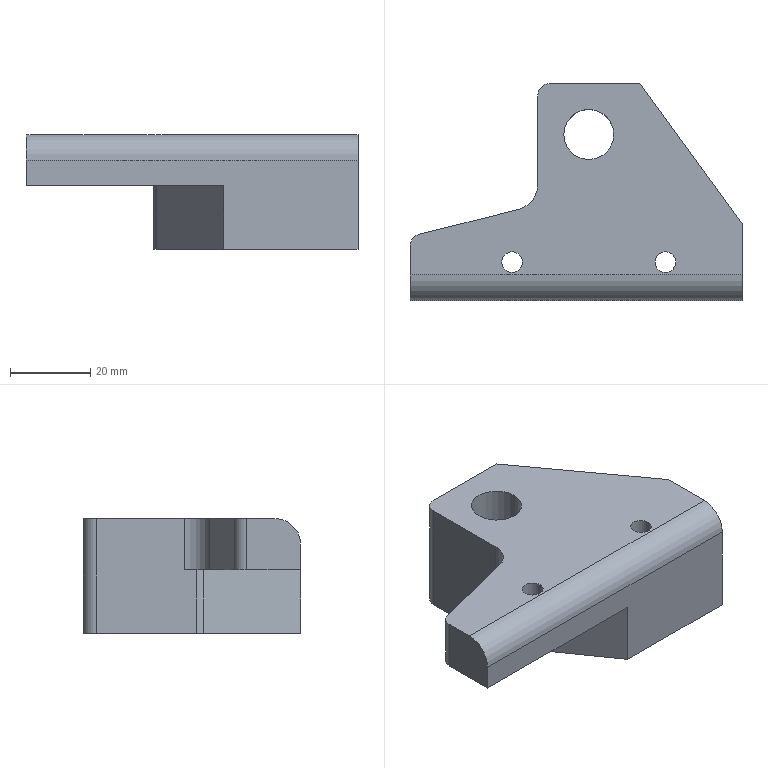Part | NX | 1 solid | 32 faces | box 82.55 x 53.975 x 28.575 mm | volume 59843 mm3 | cylinder 17 | plane 13 | cone 2 | commonest cylinder face diameters 5.16 x4 15.875 x4 6.35 x3 4.915 x2 12.446 x2 12.7 x2
STEP:
#1=CARTESIAN_POINT('',(-7.938,-17.462,0.));
#2=VERTEX_POINT('',#1);
#3=CARTESIAN_POINT('',(-23.812,-17.462,0.));
#4=VERTEX_POINT('',#3);
#5=CARTESIAN_POINT('',(-15.875,-17.462,0.));
#6=DIRECTION('',(0.,0.,-1.));
#7=DIRECTION('',(-1.,0.,0.));
#8=AXIS2_PLACEMENT_3D('',#5,#6,#7);
#9=CIRCLE('',#8,7.938);
#10=EDGE_CURVE('',#2,#4,#9,.T.);
#11=ORIENTED_EDGE('',*,*,#10,.F.);
#12=CARTESIAN_POINT('',(-7.938,-17.462,-6.35));
#13=VERTEX_POINT('',#12);
#14=CARTESIAN_POINT('',(-7.938,-17.462,0.));
#15=DIRECTION('',(0.,0.,-1.));
#16=VECTOR('',#15,1000.);
#17=LINE('',#14,#16);
#18=EDGE_CURVE('',#2,#13,#17,.T.);
#19=ORIENTED_EDGE('',*,*,#18,.T.);
#20=CARTESIAN_POINT('',(-23.812,-17.462,-6.35));
#21=VERTEX_POINT('',#20);
#22=CARTESIAN_POINT('',(-15.875,-17.462,-6.35));
#23=DIRECTION('',(0.,0.,-1.));
#24=DIRECTION('',(-1.,0.,0.));
#25=AXIS2_PLACEMENT_3D('',#22,#23,#24);
#26=CIRCLE('',#25,7.938);
#27=EDGE_CURVE('',#13,#21,#26,.T.);
#28=ORIENTED_EDGE('',*,*,#27,.T.);
#29=CARTESIAN_POINT('',(-23.812,-17.462,0.));
#30=DIRECTION('',(0.,0.,-1.));
#31=VECTOR('',#30,1000.);
#32=LINE('',#29,#31);
#33=EDGE_CURVE('',#4,#21,#32,.T.);
#34=ORIENTED_EDGE('',*,*,#33,.F.);
#35=EDGE_LOOP('',(#11,#19,#28,#34));
#36=FACE_BOUND('',#35,.T.);
#37=CARTESIAN_POINT('',(-15.875,-17.462,0.));
#38=DIRECTION('',(0.,0.,-1.));
#39=DIRECTION('',(1.,0.,0.));
#40=AXIS2_PLACEMENT_3D('',#37,#38,#39);
#41=CYLINDRICAL_SURFACE('',#40,7.938);
#42=ADVANCED_FACE('',(#36),#41,.F.);
#43=CARTESIAN_POINT('',(30.163,-17.462,0.));
#44=VERTEX_POINT('',#43);
#45=CARTESIAN_POINT('',(14.287,-17.462,0.));
#46=VERTEX_POINT('',#45);
#47=CARTESIAN_POINT('',(22.225,-17.462,0.));
#48=DIRECTION('',(0.,0.,-1.));
#49=DIRECTION('',(-1.,0.,0.));
#50=AXIS2_PLACEMENT_3D('',#47,#48,#49);
#51=CIRCLE('',#50,7.938);
#52=EDGE_CURVE('',#44,#46,#51,.T.);
#53=ORIENTED_EDGE('',*,*,#52,.F.);
#54=CARTESIAN_POINT('',(30.163,-17.462,-22.225));
#55=VERTEX_POINT('',#54);
#56=CARTESIAN_POINT('',(30.163,-17.462,0.));
#57=DIRECTION('',(0.,0.,-1.));
#58=VECTOR('',#57,1000.);
#59=LINE('',#56,#58);
#60=EDGE_CURVE('',#44,#55,#59,.T.);
#61=ORIENTED_EDGE('',*,*,#60,.T.);
#62=CARTESIAN_POINT('',(14.287,-17.462,-22.225));
#63=VERTEX_POINT('',#62);
#64=CARTESIAN_POINT('',(22.225,-17.462,-22.225));
#65=DIRECTION('',(0.,0.,-1.));
#66=DIRECTION('',(-1.,0.,0.));
#67=AXIS2_PLACEMENT_3D('',#64,#65,#66);
#68=CIRCLE('',#67,7.938);
#69=EDGE_CURVE('',#55,#63,#68,.T.);
#70=ORIENTED_EDGE('',*,*,#69,.T.);
#71=CARTESIAN_POINT('',(14.287,-17.462,0.));
#72=DIRECTION('',(0.,0.,-1.));
#73=VECTOR('',#72,1000.);
#74=LINE('',#71,#73);
#75=EDGE_CURVE('',#46,#63,#74,.T.);
#76=ORIENTED_EDGE('',*,*,#75,.F.);
#77=EDGE_LOOP('',(#53,#61,#70,#76));
#78=FACE_BOUND('',#77,.T.);
#79=CARTESIAN_POINT('',(22.225,-17.462,0.));
#80=DIRECTION('',(0.,0.,-1.));
#81=DIRECTION('',(1.,0.,0.));
#82=AXIS2_PLACEMENT_3D('',#79,#80,#81);
#83=CYLINDRICAL_SURFACE('',#82,7.938);
#84=ADVANCED_FACE('',(#78),#83,.F.);
#85=CARTESIAN_POINT('',(30.15,-1.587,-8.048));
#86=VERTEX_POINT('',#85);
#87=CARTESIAN_POINT('',(27.692,-1.587,-9.525));
#88=VERTEX_POINT('',#87);
#89=CARTESIAN_POINT('',(27.692,-1.587,-9.525));
#90=DIRECTION('',(-0.8572,0.,-0.515));
#91=VECTOR('',#90,1000.);
#92=LINE('',#89,#91);
#93=EDGE_CURVE('',#86,#88,#92,.T.);
#94=ORIENTED_EDGE('',*,*,#93,.F.);
#95=CARTESIAN_POINT('',(32.607,-1.587,-9.525));
#96=VERTEX_POINT('',#95);
#97=CARTESIAN_POINT('',(32.607,-1.587,-9.525));
#98=DIRECTION('',(0.8572,0.,-0.515));
#99=VECTOR('',#98,1000.);
#100=LINE('',#97,#99);
#101=EDGE_CURVE('',#86,#96,#100,.T.);
#102=ORIENTED_EDGE('',*,*,#101,.T.);
#103=CARTESIAN_POINT('',(30.15,-1.587,-9.525));
#104=DIRECTION('',(0.,0.,-1.));
#105=DIRECTION('',(-1.,0.,0.));
#106=AXIS2_PLACEMENT_3D('',#103,#104,#105);
#107=CIRCLE('',#106,2.457);
#108=EDGE_CURVE('',#96,#88,#107,.T.);
#109=ORIENTED_EDGE('',*,*,#108,.T.);
#110=EDGE_LOOP('',(#94,#102,#109));
#111=FACE_BOUND('',#110,.T.);
#112=CARTESIAN_POINT('',(30.15,-1.587,-9.525));
#113=DIRECTION('',(0.,0.,-1.));
#114=DIRECTION('',(1.,0.,0.));
#115=AXIS2_PLACEMENT_3D('',#112,#113,#114);
#116=CONICAL_SURFACE('',#115,2.457,1.03);
#117=ADVANCED_FACE('',(#111),#116,.F.);
#118=ORIENTED_EDGE('',*,*,#108,.F.);
#119=CARTESIAN_POINT('',(32.607,-1.587,-22.225));
#120=VERTEX_POINT('',#119);
#121=CARTESIAN_POINT('',(32.607,-1.587,-22.225));
#122=DIRECTION('',(0.,0.,-1.));
#123=VECTOR('',#122,1000.);
#124=LINE('',#121,#123);
#125=EDGE_CURVE('',#96,#120,#124,.T.);
#126=ORIENTED_EDGE('',*,*,#125,.T.);
#127=CARTESIAN_POINT('',(27.692,-1.587,-22.225));
#128=VERTEX_POINT('',#127);
#129=CARTESIAN_POINT('',(30.15,-1.587,-22.225));
#130=DIRECTION('',(0.,0.,-1.));
#131=DIRECTION('',(-1.,0.,0.));
#132=AXIS2_PLACEMENT_3D('',#129,#130,#131);
#133=CIRCLE('',#132,2.457);
#134=EDGE_CURVE('',#120,#128,#133,.T.);
#135=ORIENTED_EDGE('',*,*,#134,.T.);
#136=CARTESIAN_POINT('',(27.692,-1.587,-22.225));
#137=DIRECTION('',(0.,0.,-1.));
#138=VECTOR('',#137,1000.);
#139=LINE('',#136,#138);
#140=EDGE_CURVE('',#88,#128,#139,.T.);
#141=ORIENTED_EDGE('',*,*,#140,.F.);
#142=EDGE_LOOP('',(#118,#126,#135,#141));
#143=FACE_BOUND('',#142,.T.);
#144=CARTESIAN_POINT('',(30.15,-1.587,-22.225));
#145=DIRECTION('',(0.,0.,-1.));
#146=DIRECTION('',(1.,0.,0.));
#147=AXIS2_PLACEMENT_3D('',#144,#145,#146);
#148=CYLINDRICAL_SURFACE('',#147,2.457);
#149=ADVANCED_FACE('',(#143),#148,.F.);
#150=CARTESIAN_POINT('',(9.398,14.287,6.35));
#151=VERTEX_POINT('',#150);
#152=CARTESIAN_POINT('',(-3.048,14.287,6.35));
#153=VERTEX_POINT('',#152);
#154=CARTESIAN_POINT('',(3.175,14.287,6.35));
#155=DIRECTION('',(0.,0.,-1.));
#156=DIRECTION('',(-1.,0.,0.));
#157=AXIS2_PLACEMENT_3D('',#154,#155,#156);
#158=CIRCLE('',#157,6.223);
#159=EDGE_CURVE('',#151,#153,#158,.T.);
#160=ORIENTED_EDGE('',*,*,#159,.F.);
#161=CARTESIAN_POINT('',(9.398,14.287,-22.225));
#162=VERTEX_POINT('',#161);
#163=CARTESIAN_POINT('',(9.398,14.287,6.35));
#164=DIRECTION('',(0.,0.,-1.));
#165=VECTOR('',#164,1000.);
#166=LINE('',#163,#165);
#167=EDGE_CURVE('',#151,#162,#166,.T.);
#168=ORIENTED_EDGE('',*,*,#167,.T.);
#169=CARTESIAN_POINT('',(-3.048,14.287,-22.225));
#170=VERTEX_POINT('',#169);
#171=CARTESIAN_POINT('',(3.175,14.287,-22.225));
#172=DIRECTION('',(0.,0.,-1.));
#173=DIRECTION('',(-1.,0.,0.));
#174=AXIS2_PLACEMENT_3D('',#171,#172,#173);
#175=CIRCLE('',#174,6.223);
#176=EDGE_CURVE('',#162,#170,#175,.T.);
#177=ORIENTED_EDGE('',*,*,#176,.T.);
#178=CARTESIAN_POINT('',(-3.048,14.287,6.35));
#179=DIRECTION('',(0.,0.,-1.));
#180=VECTOR('',#179,1000.);
#181=LINE('',#178,#180);
#182=EDGE_CURVE('',#153,#170,#181,.T.);
#183=ORIENTED_EDGE('',*,*,#182,.F.);
#184=EDGE_LOOP('',(#160,#168,#177,#183));
#185=FACE_BOUND('',#184,.T.);
#186=CARTESIAN_POINT('',(3.175,14.287,6.35));
#187=DIRECTION('',(0.,0.,-1.));
#188=DIRECTION('',(1.,0.,0.));
#189=AXIS2_PLACEMENT_3D('',#186,#187,#188);
#190=CYLINDRICAL_SURFACE('',#189,6.223);
#191=ADVANCED_FACE('',(#185),#190,.F.);
#192=CARTESIAN_POINT('',(24.805,-17.462,6.35));
#193=VERTEX_POINT('',#192);
#194=CARTESIAN_POINT('',(19.645,-17.462,6.35));
#195=VERTEX_POINT('',#194);
#196=CARTESIAN_POINT('',(22.225,-17.462,6.35));
#197=DIRECTION('',(0.,0.,-1.));
#198=DIRECTION('',(-1.,0.,0.));
#199=AXIS2_PLACEMENT_3D('',#196,#197,#198);
#200=CIRCLE('',#199,2.58);
#201=EDGE_CURVE('',#193,#195,#200,.T.);
#202=ORIENTED_EDGE('',*,*,#201,.F.);
#203=CARTESIAN_POINT('',(24.805,-17.462,0.));
#204=VERTEX_POINT('',#203);
#205=CARTESIAN_POINT('',(24.805,-17.462,-22.225));
#206=DIRECTION('',(0.,0.,-1.));
#207=VECTOR('',#206,1000.);
#208=LINE('',#205,#207);
#209=EDGE_CURVE('',#193,#204,#208,.T.);
#210=ORIENTED_EDGE('',*,*,#209,.T.);
#211=CARTESIAN_POINT('',(19.645,-17.462,0.));
#212=VERTEX_POINT('',#211);
#213=CARTESIAN_POINT('',(22.225,-17.462,0.));
#214=DIRECTION('',(0.,0.,1.));
#215=DIRECTION('',(-1.,0.,0.));
#216=AXIS2_PLACEMENT_3D('',#213,#214,#215);
#217=CIRCLE('',#216,2.58);
#218=EDGE_CURVE('',#212,#204,#217,.T.);
#219=ORIENTED_EDGE('',*,*,#218,.F.);
#220=CARTESIAN_POINT('',(19.645,-17.462,-22.225));
#221=DIRECTION('',(0.,0.,-1.));
#222=VECTOR('',#221,1000.);
#223=LINE('',#220,#222);
#224=EDGE_CURVE('',#195,#212,#223,.T.);
#225=ORIENTED_EDGE('',*,*,#224,.F.);
#226=EDGE_LOOP('',(#202,#210,#219,#225));
#227=FACE_BOUND('',#226,.T.);
#228=CARTESIAN_POINT('',(22.225,-17.462,-22.225));
#229=DIRECTION('',(0.,0.,-1.));
#230=DIRECTION('',(1.,0.,0.));
#231=AXIS2_PLACEMENT_3D('',#228,#229,#230);
#232=CYLINDRICAL_SURFACE('',#231,2.58);
#233=ADVANCED_FACE('',(#227),#232,.F.);
#234=CARTESIAN_POINT('',(-13.295,-17.462,6.35));
#235=VERTEX_POINT('',#234);
#236=CARTESIAN_POINT('',(-18.455,-17.462,6.35));
#237=VERTEX_POINT('',#236);
#238=CARTESIAN_POINT('',(-15.875,-17.462,6.35));
#239=DIRECTION('',(0.,0.,-1.));
#240=DIRECTION('',(-1.,0.,0.));
#241=AXIS2_PLACEMENT_3D('',#238,#239,#240);
#242=CIRCLE('',#241,2.58);
#243=EDGE_CURVE('',#235,#237,#242,.T.);
#244=ORIENTED_EDGE('',*,*,#243,.F.);
#245=CARTESIAN_POINT('',(-13.295,-17.462,0.));
#246=VERTEX_POINT('',#245);
#247=CARTESIAN_POINT('',(-13.295,-17.462,-22.225));
#248=DIRECTION('',(0.,0.,-1.));
#249=VECTOR('',#248,1000.);
#250=LINE('',#247,#249);
#251=EDGE_CURVE('',#235,#246,#250,.T.);
#252=ORIENTED_EDGE('',*,*,#251,.T.);
#253=CARTESIAN_POINT('',(-18.455,-17.462,0.));
#254=VERTEX_POINT('',#253);
#255=CARTESIAN_POINT('',(-15.875,-17.462,0.));
#256=DIRECTION('',(0.,0.,1.));
#257=DIRECTION('',(-1.,0.,0.));
#258=AXIS2_PLACEMENT_3D('',#255,#256,#257);
#259=CIRCLE('',#258,2.58);
#260=EDGE_CURVE('',#254,#246,#259,.T.);
#261=ORIENTED_EDGE('',*,*,#260,.F.);
#262=CARTESIAN_POINT('',(-18.455,-17.462,-22.225));
#263=DIRECTION('',(0.,0.,-1.));
#264=VECTOR('',#263,1000.);
#265=LINE('',#262,#264);
#266=EDGE_CURVE('',#237,#254,#265,.T.);
#267=ORIENTED_EDGE('',*,*,#266,.F.);
#268=EDGE_LOOP('',(#244,#252,#261,#267));
#269=FACE_BOUND('',#268,.T.);
#270=CARTESIAN_POINT('',(-15.875,-17.462,-22.225));
#271=DIRECTION('',(0.,0.,-1.));
#272=DIRECTION('',(1.,0.,0.));
#273=AXIS2_PLACEMENT_3D('',#270,#271,#272);
#274=CYLINDRICAL_SURFACE('',#273,2.58);
#275=ADVANCED_FACE('',(#269),#274,.F.);
#276=ORIENTED_EDGE('',*,*,#251,.F.);
#277=CARTESIAN_POINT('',(-15.875,-17.462,6.35));
#278=DIRECTION('',(0.,0.,-1.));
#279=DIRECTION('',(-1.,0.,0.));
#280=AXIS2_PLACEMENT_3D('',#277,#278,#279);
#281=CIRCLE('',#280,2.58);
#282=EDGE_CURVE('',#237,#235,#281,.T.);
#283=ORIENTED_EDGE('',*,*,#282,.F.);
#284=ORIENTED_EDGE('',*,*,#266,.T.);
#285=CARTESIAN_POINT('',(-15.875,-17.462,0.));
#286=DIRECTION('',(0.,0.,1.));
#287=DIRECTION('',(-1.,0.,0.));
#288=AXIS2_PLACEMENT_3D('',#285,#286,#287);
#289=CIRCLE('',#288,2.58);
#290=EDGE_CURVE('',#246,#254,#289,.T.);
#291=ORIENTED_EDGE('',*,*,#290,.F.);
#292=EDGE_LOOP('',(#276,#283,#284,#291));
#293=FACE_BOUND('',#292,.T.);
#294=CARTESIAN_POINT('',(-15.875,-17.462,-22.225));
#295=DIRECTION('',(0.,0.,-1.));
#296=DIRECTION('',(1.,0.,0.));
#297=AXIS2_PLACEMENT_3D('',#294,#295,#296);
#298=CYLINDRICAL_SURFACE('',#297,2.58);
#299=ADVANCED_FACE('',(#293),#298,.F.);
#300=ORIENTED_EDGE('',*,*,#209,.F.);
#301=CARTESIAN_POINT('',(22.225,-17.462,6.35));
#302=DIRECTION('',(0.,0.,-1.));
#303=DIRECTION('',(-1.,0.,0.));
#304=AXIS2_PLACEMENT_3D('',#301,#302,#303);
#305=CIRCLE('',#304,2.58);
#306=EDGE_CURVE('',#195,#193,#305,.T.);
#307=ORIENTED_EDGE('',*,*,#306,.F.);
#308=ORIENTED_EDGE('',*,*,#224,.T.);
#309=CARTESIAN_POINT('',(22.225,-17.462,0.));
#310=DIRECTION('',(0.,0.,1.));
#311=DIRECTION('',(-1.,0.,0.));
#312=AXIS2_PLACEMENT_3D('',#309,#310,#311);
#313=CIRCLE('',#312,2.58);
#314=EDGE_CURVE('',#204,#212,#313,.T.);
#315=ORIENTED_EDGE('',*,*,#314,.F.);
#316=EDGE_LOOP('',(#300,#307,#308,#315));
#317=FACE_BOUND('',#316,.T.);
#318=CARTESIAN_POINT('',(22.225,-17.462,-22.225));
#319=DIRECTION('',(0.,0.,-1.));
#320=DIRECTION('',(1.,0.,0.));
#321=AXIS2_PLACEMENT_3D('',#318,#319,#320);
#322=CYLINDRICAL_SURFACE('',#321,2.58);
#323=ADVANCED_FACE('',(#317),#322,.F.);
#324=CARTESIAN_POINT('',(41.275,-7.938,6.35));
#325=VERTEX_POINT('',#324);
#326=CARTESIAN_POINT('',(41.275,-7.938,-22.225));
#327=VERTEX_POINT('',#326);
#328=CARTESIAN_POINT('',(41.275,-7.938,6.35));
#329=DIRECTION('',(0.,0.,-1.));
#330=VECTOR('',#329,1000.);
#331=LINE('',#328,#330);
#332=EDGE_CURVE('',#325,#327,#331,.T.);
#333=ORIENTED_EDGE('',*,*,#332,.T.);
#334=CARTESIAN_POINT('',(15.875,26.988,-22.225));
#335=VERTEX_POINT('',#334);
#336=CARTESIAN_POINT('',(41.275,-7.938,-22.225));
#337=DIRECTION('',(-0.5882,0.8087,0.));
#338=VECTOR('',#337,1000.);
#339=LINE('',#336,#338);
#340=EDGE_CURVE('',#327,#335,#339,.T.);
#341=ORIENTED_EDGE('',*,*,#340,.T.);
#342=CARTESIAN_POINT('',(15.875,26.988,6.35));
#343=VERTEX_POINT('',#342);
#344=CARTESIAN_POINT('',(15.875,26.988,6.35));
#345=DIRECTION('',(0.,0.,-1.));
#346=VECTOR('',#345,1000.);
#347=LINE('',#344,#346);
#348=EDGE_CURVE('',#343,#335,#347,.T.);
#349=ORIENTED_EDGE('',*,*,#348,.F.);
#350=CARTESIAN_POINT('',(41.275,-7.938,6.35));
#351=DIRECTION('',(-0.5882,0.8087,0.));
#352=VECTOR('',#351,1000.);
#353=LINE('',#350,#352);
#354=EDGE_CURVE('',#325,#343,#353,.T.);
#355=ORIENTED_EDGE('',*,*,#354,.F.);
#356=EDGE_LOOP('',(#333,#341,#349,#355));
#357=FACE_BOUND('',#356,.T.);
#358=CARTESIAN_POINT('',(41.275,-7.938,6.35));
#359=DIRECTION('',(-0.8087,-0.5882,0.));
#360=DIRECTION('',(-0.5882,0.8087,0.));
#361=AXIS2_PLACEMENT_3D('',#358,#359,#360);
#362=PLANE('',#361);
#363=ADVANCED_FACE('',(#357),#362,.F.);
#364=ORIENTED_EDGE('',*,*,#348,.T.);
#365=CARTESIAN_POINT('',(-6.35,26.988,-22.225));
#366=VERTEX_POINT('',#365);
#367=CARTESIAN_POINT('',(15.875,26.988,-22.225));
#368=DIRECTION('',(-1.,0.,0.));
#369=VECTOR('',#368,1000.);
#370=LINE('',#367,#369);
#371=EDGE_CURVE('',#335,#366,#370,.T.);
#372=ORIENTED_EDGE('',*,*,#371,.T.);
#373=CARTESIAN_POINT('',(-6.35,26.988,6.35));
#374=VERTEX_POINT('',#373);
#375=CARTESIAN_POINT('',(-6.35,26.988,6.35));
#376=DIRECTION('',(0.,0.,1.));
#377=VECTOR('',#376,1000.);
#378=LINE('',#375,#377);
#379=EDGE_CURVE('',#366,#374,#378,.T.);
#380=ORIENTED_EDGE('',*,*,#379,.T.);
#381=CARTESIAN_POINT('',(15.875,26.988,6.35));
#382=DIRECTION('',(-1.,0.,0.));
#383=VECTOR('',#382,1000.);
#384=LINE('',#381,#383);
#385=EDGE_CURVE('',#343,#374,#384,.T.);
#386=ORIENTED_EDGE('',*,*,#385,.F.);
#387=EDGE_LOOP('',(#364,#372,#380,#386));
#388=FACE_BOUND('',#387,.T.);
#389=CARTESIAN_POINT('',(15.875,26.988,6.35));
#390=DIRECTION('',(0.,-1.,0.));
#391=DIRECTION('',(-1.,0.,0.));
#392=AXIS2_PLACEMENT_3D('',#389,#390,#391);
#393=PLANE('',#392);
#394=ADVANCED_FACE('',(#388),#393,.F.);
#395=CARTESIAN_POINT('',(-9.525,23.812,6.35));
#396=VERTEX_POINT('',#395);
#397=CARTESIAN_POINT('',(-9.525,23.812,-22.225));
#398=VERTEX_POINT('',#397);
#399=CARTESIAN_POINT('',(-9.525,23.812,6.35));
#400=DIRECTION('',(0.,0.,-1.));
#401=VECTOR('',#400,1000.);
#402=LINE('',#399,#401);
#403=EDGE_CURVE('',#396,#398,#402,.T.);
#404=ORIENTED_EDGE('',*,*,#403,.T.);
#405=CARTESIAN_POINT('',(-9.525,-1.047,-22.225));
#406=VERTEX_POINT('',#405);
#407=CARTESIAN_POINT('',(-9.525,23.812,-22.225));
#408=DIRECTION('',(0.,-1.,0.));
#409=VECTOR('',#408,1000.);
#410=LINE('',#407,#409);
#411=EDGE_CURVE('',#398,#406,#410,.T.);
#412=ORIENTED_EDGE('',*,*,#411,.T.);
#413=CARTESIAN_POINT('',(-9.525,-1.047,-6.35));
#414=VERTEX_POINT('',#413);
#415=CARTESIAN_POINT('',(-9.525,-1.047,-22.225));
#416=DIRECTION('',(0.,0.,1.));
#417=VECTOR('',#416,1000.);
#418=LINE('',#415,#417);
#419=EDGE_CURVE('',#406,#414,#418,.T.);
#420=ORIENTED_EDGE('',*,*,#419,.T.);
#421=CARTESIAN_POINT('',(-9.525,1.794,-6.35));
#422=VERTEX_POINT('',#421);
#423=CARTESIAN_POINT('',(-9.525,6.863,-6.35));
#424=DIRECTION('',(0.,-1.,0.));
#425=VECTOR('',#424,1000.);
#426=LINE('',#423,#425);
#427=EDGE_CURVE('',#422,#414,#426,.T.);
#428=ORIENTED_EDGE('',*,*,#427,.F.);
#429=CARTESIAN_POINT('',(-9.525,1.794,6.35));
#430=VERTEX_POINT('',#429);
#431=CARTESIAN_POINT('',(-9.525,1.794,6.35));
#432=DIRECTION('',(0.,0.,1.));
#433=VECTOR('',#432,1000.);
#434=LINE('',#431,#433);
#435=EDGE_CURVE('',#422,#430,#434,.T.);
#436=ORIENTED_EDGE('',*,*,#435,.T.);
#437=CARTESIAN_POINT('',(-9.525,26.988,6.35));
#438=DIRECTION('',(0.,-1.,0.));
#439=VECTOR('',#438,1000.);
#440=LINE('',#437,#439);
#441=EDGE_CURVE('',#396,#430,#440,.T.);
#442=ORIENTED_EDGE('',*,*,#441,.F.);
#443=EDGE_LOOP('',(#404,#412,#420,#428,#436,#442));
#444=FACE_BOUND('',#443,.T.);
#445=CARTESIAN_POINT('',(-9.525,26.988,6.35));
#446=DIRECTION('',(1.,0.,0.));
#447=DIRECTION('',(0.,-1.,0.));
#448=AXIS2_PLACEMENT_3D('',#445,#446,#447);
#449=PLANE('',#448);
#450=ADVANCED_FACE('',(#444),#449,.F.);
#451=CARTESIAN_POINT('',(-14.333,-4.366,6.35));
#452=VERTEX_POINT('',#451);
#453=CARTESIAN_POINT('',(-38.871,-10.511,6.35));
#454=VERTEX_POINT('',#453);
#455=CARTESIAN_POINT('',(-9.525,-3.162,6.35));
#456=DIRECTION('',(-0.9701,-0.2429,0.));
#457=VECTOR('',#456,1000.);
#458=LINE('',#455,#457);
#459=EDGE_CURVE('',#452,#454,#458,.T.);
#460=ORIENTED_EDGE('',*,*,#459,.F.);
#461=CARTESIAN_POINT('',(-14.333,-4.366,-6.35));
#462=VERTEX_POINT('',#461);
#463=CARTESIAN_POINT('',(-14.333,-4.366,-6.35));
#464=DIRECTION('',(0.,0.,-1.));
#465=VECTOR('',#464,1000.);
#466=LINE('',#463,#465);
#467=EDGE_CURVE('',#452,#462,#466,.T.);
#468=ORIENTED_EDGE('',*,*,#467,.T.);
#469=CARTESIAN_POINT('',(-38.871,-10.511,-6.35));
#470=VERTEX_POINT('',#469);
#471=CARTESIAN_POINT('',(-9.525,-3.162,-6.35));
#472=DIRECTION('',(-0.9701,-0.2429,0.));
#473=VECTOR('',#472,1000.);
#474=LINE('',#471,#473);
#475=EDGE_CURVE('',#462,#470,#474,.T.);
#476=ORIENTED_EDGE('',*,*,#475,.T.);
#477=CARTESIAN_POINT('',(-38.871,-10.511,6.35));
#478=DIRECTION('',(0.,0.,1.));
#479=VECTOR('',#478,1000.);
#480=LINE('',#477,#479);
#481=EDGE_CURVE('',#470,#454,#480,.T.);
#482=ORIENTED_EDGE('',*,*,#481,.T.);
#483=EDGE_LOOP('',(#460,#468,#476,#482));
#484=FACE_BOUND('',#483,.T.);
#485=CARTESIAN_POINT('',(-9.525,-3.162,6.35));
#486=DIRECTION('',(0.2429,-0.9701,0.));
#487=DIRECTION('',(-0.9701,-0.2429,0.));
#488=AXIS2_PLACEMENT_3D('',#485,#486,#487);
#489=PLANE('',#488);
#490=ADVANCED_FACE('',(#484),#489,.F.);
#491=CARTESIAN_POINT('',(-41.275,-26.988,0.));
#492=VERTEX_POINT('',#491);
#493=CARTESIAN_POINT('',(-41.275,-26.988,-6.35));
#494=VERTEX_POINT('',#493);
#495=CARTESIAN_POINT('',(-41.275,-26.988,6.35));
#496=DIRECTION('',(0.,0.,-1.));
#497=VECTOR('',#496,1000.);
#498=LINE('',#495,#497);
#499=EDGE_CURVE('',#492,#494,#498,.T.);
#500=ORIENTED_EDGE('',*,*,#499,.F.);
#501=CARTESIAN_POINT('',(-41.275,-20.637,6.35));
#502=VERTEX_POINT('',#501);
#503=CARTESIAN_POINT('',(-41.275,-20.637,0.));
#504=DIRECTION('',(-1.,0.,0.));
#505=DIRECTION('',(0.,0.,-1.));
#506=AXIS2_PLACEMENT_3D('',#503,#504,#505);
#507=CIRCLE('',#506,6.35);
#508=EDGE_CURVE('',#492,#502,#507,.T.);
#509=ORIENTED_EDGE('',*,*,#508,.T.);
#510=CARTESIAN_POINT('',(-41.275,-13.591,6.35));
#511=VERTEX_POINT('',#510);
#512=CARTESIAN_POINT('',(-41.275,-11.113,6.35));
#513=DIRECTION('',(0.,-1.,0.));
#514=VECTOR('',#513,1000.);
#515=LINE('',#512,#514);
#516=EDGE_CURVE('',#511,#502,#515,.T.);
#517=ORIENTED_EDGE('',*,*,#516,.F.);
#518=CARTESIAN_POINT('',(-41.275,-13.591,-6.35));
#519=VERTEX_POINT('',#518);
#520=CARTESIAN_POINT('',(-41.275,-13.591,6.35));
#521=DIRECTION('',(0.,0.,-1.));
#522=VECTOR('',#521,1000.);
#523=LINE('',#520,#522);
#524=EDGE_CURVE('',#511,#519,#523,.T.);
#525=ORIENTED_EDGE('',*,*,#524,.T.);
#526=CARTESIAN_POINT('',(-41.275,-11.113,-6.35));
#527=DIRECTION('',(0.,-1.,0.));
#528=VECTOR('',#527,1000.);
#529=LINE('',#526,#528);
#530=EDGE_CURVE('',#519,#494,#529,.T.);
#531=ORIENTED_EDGE('',*,*,#530,.T.);
#532=EDGE_LOOP('',(#500,#509,#517,#525,#531));
#533=FACE_BOUND('',#532,.T.);
#534=CARTESIAN_POINT('',(-41.275,-11.113,6.35));
#535=DIRECTION('',(1.,0.,0.));
#536=DIRECTION('',(0.,0.,1.));
#537=AXIS2_PLACEMENT_3D('',#534,#535,#536);
#538=PLANE('',#537);
#539=ADVANCED_FACE('',(#533),#538,.F.);
#540=CARTESIAN_POINT('',(41.275,-26.988,0.));
#541=VERTEX_POINT('',#540);
#542=CARTESIAN_POINT('',(41.275,-26.988,-22.225));
#543=VERTEX_POINT('',#542);
#544=CARTESIAN_POINT('',(41.275,-26.988,6.35));
#545=DIRECTION('',(0.,0.,-1.));
#546=VECTOR('',#545,1000.);
#547=LINE('',#544,#546);
#548=EDGE_CURVE('',#541,#543,#547,.T.);
#549=ORIENTED_EDGE('',*,*,#548,.F.);
#550=CARTESIAN_POINT('',(-41.275,-26.988,0.));
#551=DIRECTION('',(-1.,0.,0.));
#552=VECTOR('',#551,1000.);
#553=LINE('',#550,#552);
#554=EDGE_CURVE('',#541,#492,#553,.T.);
#555=ORIENTED_EDGE('',*,*,#554,.T.);
#556=ORIENTED_EDGE('',*,*,#499,.T.);
#557=CARTESIAN_POINT('',(7.938,-26.988,-6.35));
#558=VERTEX_POINT('',#557);
#559=CARTESIAN_POINT('',(-41.275,-26.988,-6.35));
#560=DIRECTION('',(1.,0.,0.));
#561=VECTOR('',#560,1000.);
#562=LINE('',#559,#561);
#563=EDGE_CURVE('',#494,#558,#562,.T.);
#564=ORIENTED_EDGE('',*,*,#563,.T.);
#565=CARTESIAN_POINT('',(7.938,-26.988,-22.225));
#566=VERTEX_POINT('',#565);
#567=CARTESIAN_POINT('',(7.938,-26.988,-22.225));
#568=DIRECTION('',(0.,0.,1.));
#569=VECTOR('',#568,1000.);
#570=LINE('',#567,#569);
#571=EDGE_CURVE('',#566,#558,#570,.T.);
#572=ORIENTED_EDGE('',*,*,#571,.F.);
#573=CARTESIAN_POINT('',(7.938,-26.988,-22.225));
#574=DIRECTION('',(1.,0.,0.));
#575=VECTOR('',#574,1000.);
#576=LINE('',#573,#575);
#577=EDGE_CURVE('',#566,#543,#576,.T.);
#578=ORIENTED_EDGE('',*,*,#577,.T.);
#579=EDGE_LOOP('',(#549,#555,#556,#564,#572,#578));
#580=FACE_BOUND('',#579,.T.);
#581=CARTESIAN_POINT('',(-41.275,-26.988,6.35));
#582=DIRECTION('',(0.,1.,0.));
#583=DIRECTION('',(0.,0.,-1.));
#584=AXIS2_PLACEMENT_3D('',#581,#582,#583);
#585=PLANE('',#584);
#586=ADVANCED_FACE('',(#580),#585,.F.);
#587=CARTESIAN_POINT('',(41.275,-20.637,6.35));
#588=VERTEX_POINT('',#587);
#589=CARTESIAN_POINT('',(41.275,-26.988,6.35));
#590=DIRECTION('',(0.,1.,0.));
#591=VECTOR('',#590,1000.);
#592=LINE('',#589,#591);
#593=EDGE_CURVE('',#588,#325,#592,.T.);
#594=ORIENTED_EDGE('',*,*,#593,.F.);
#595=CARTESIAN_POINT('',(41.275,-20.637,0.));
#596=DIRECTION('',(1.,0.,0.));
#597=DIRECTION('',(0.,-1.,0.));
#598=AXIS2_PLACEMENT_3D('',#595,#596,#597);
#599=CIRCLE('',#598,6.35);
#600=EDGE_CURVE('',#588,#541,#599,.T.);
#601=ORIENTED_EDGE('',*,*,#600,.T.);
#602=ORIENTED_EDGE('',*,*,#548,.T.);
#603=CARTESIAN_POINT('',(41.275,-26.988,-22.225));
#604=DIRECTION('',(0.,1.,0.));
#605=VECTOR('',#604,1000.);
#606=LINE('',#603,#605);
#607=EDGE_CURVE('',#543,#327,#606,.T.);
#608=ORIENTED_EDGE('',*,*,#607,.T.);
#609=ORIENTED_EDGE('',*,*,#332,.F.);
#610=EDGE_LOOP('',(#594,#601,#602,#608,#609));
#611=FACE_BOUND('',#610,.T.);
#612=CARTESIAN_POINT('',(41.275,-26.988,6.35));
#613=DIRECTION('',(-1.,0.,0.));
#614=DIRECTION('',(0.,1.,0.));
#615=AXIS2_PLACEMENT_3D('',#612,#613,#614);
#616=PLANE('',#615);
#617=ADVANCED_FACE('',(#611),#616,.F.);
#618=ORIENTED_EDGE('',*,*,#306,.T.);
#619=ORIENTED_EDGE('',*,*,#201,.T.);
#620=EDGE_LOOP('',(#618,#619));
#621=FACE_BOUND('',#620,.T.);
#622=ORIENTED_EDGE('',*,*,#282,.T.);
#623=ORIENTED_EDGE('',*,*,#243,.T.);
#624=EDGE_LOOP('',(#622,#623));
#625=FACE_BOUND('',#624,.T.);
#626=CARTESIAN_POINT('',(3.175,14.287,6.35));
#627=DIRECTION('',(0.,0.,-1.));
#628=DIRECTION('',(-1.,0.,0.));
#629=AXIS2_PLACEMENT_3D('',#626,#627,#628);
#630=CIRCLE('',#629,6.223);
#631=EDGE_CURVE('',#153,#151,#630,.T.);
#632=ORIENTED_EDGE('',*,*,#631,.T.);
#633=ORIENTED_EDGE('',*,*,#159,.T.);
#634=EDGE_LOOP('',(#632,#633));
#635=FACE_BOUND('',#634,.T.);
#636=ORIENTED_EDGE('',*,*,#516,.T.);
#637=CARTESIAN_POINT('',(41.275,-20.637,6.35));
#638=DIRECTION('',(1.,0.,0.));
#639=VECTOR('',#638,1000.);
#640=LINE('',#637,#639);
#641=EDGE_CURVE('',#502,#588,#640,.T.);
#642=ORIENTED_EDGE('',*,*,#641,.T.);
#643=ORIENTED_EDGE('',*,*,#593,.T.);
#644=ORIENTED_EDGE('',*,*,#354,.T.);
#645=ORIENTED_EDGE('',*,*,#385,.T.);
#646=CARTESIAN_POINT('',(-6.35,23.812,6.35));
#647=DIRECTION('',(0.,0.,1.));
#648=DIRECTION('',(1.,0.,0.));
#649=AXIS2_PLACEMENT_3D('',#646,#647,#648);
#650=CIRCLE('',#649,3.175);
#651=EDGE_CURVE('',#374,#396,#650,.T.);
#652=ORIENTED_EDGE('',*,*,#651,.T.);
#653=ORIENTED_EDGE('',*,*,#441,.T.);
#654=CARTESIAN_POINT('',(-15.875,1.794,6.35));
#655=DIRECTION('',(0.,0.,-1.));
#656=DIRECTION('',(1.,0.,0.));
#657=AXIS2_PLACEMENT_3D('',#654,#655,#656);
#658=CIRCLE('',#657,6.35);
#659=EDGE_CURVE('',#430,#452,#658,.T.);
#660=ORIENTED_EDGE('',*,*,#659,.T.);
#661=ORIENTED_EDGE('',*,*,#459,.T.);
#662=CARTESIAN_POINT('',(-38.1,-13.591,6.35));
#663=DIRECTION('',(0.,0.,1.));
#664=DIRECTION('',(1.,0.,0.));
#665=AXIS2_PLACEMENT_3D('',#662,#663,#664);
#666=CIRCLE('',#665,3.175);
#667=EDGE_CURVE('',#454,#511,#666,.T.);
#668=ORIENTED_EDGE('',*,*,#667,.T.);
#669=EDGE_LOOP('',(#636,#642,#643,#644,#645,#652,#653,#660,#661,#668));
#670=FACE_BOUND('',#669,.T.);
#671=CARTESIAN_POINT('',(30.511,6.863,6.35));
#672=DIRECTION('',(0.,0.,1.));
#673=DIRECTION('',(-1.,0.,0.));
#674=AXIS2_PLACEMENT_3D('',#671,#672,#673);
#675=PLANE('',#674);
#676=ADVANCED_FACE('',(#621,#625,#635,#670),#675,.T.);
#677=CARTESIAN_POINT('',(-15.875,-17.462,-6.35));
#678=DIRECTION('',(0.,0.,-1.));
#679=DIRECTION('',(-1.,0.,0.));
#680=AXIS2_PLACEMENT_3D('',#677,#678,#679);
#681=CIRCLE('',#680,7.938);
#682=EDGE_CURVE('',#21,#13,#681,.T.);
#683=ORIENTED_EDGE('',*,*,#682,.F.);
#684=ORIENTED_EDGE('',*,*,#27,.F.);
#685=EDGE_LOOP('',(#683,#684));
#686=FACE_BOUND('',#685,.T.);
#687=CARTESIAN_POINT('',(-8.951,-2.868,-6.35));
#688=VERTEX_POINT('',#687);
#689=CARTESIAN_POINT('',(-6.35,-1.047,-6.35));
#690=DIRECTION('',(0.,0.,1.));
#691=DIRECTION('',(1.,0.,0.));
#692=AXIS2_PLACEMENT_3D('',#689,#690,#691);
#693=CIRCLE('',#692,3.175);
#694=EDGE_CURVE('',#414,#688,#693,.T.);
#695=ORIENTED_EDGE('',*,*,#694,.T.);
#696=CARTESIAN_POINT('',(-0.5404,-14.88,-6.35));
#697=DIRECTION('',(0.5736,-0.8192,0.));
#698=VECTOR('',#697,1000.);
#699=LINE('',#696,#698);
#700=EDGE_CURVE('',#688,#558,#699,.T.);
#701=ORIENTED_EDGE('',*,*,#700,.T.);
#702=ORIENTED_EDGE('',*,*,#563,.F.);
#703=ORIENTED_EDGE('',*,*,#530,.F.);
#704=CARTESIAN_POINT('',(-38.1,-13.591,-6.35));
#705=DIRECTION('',(0.,0.,-1.));
#706=DIRECTION('',(1.,0.,0.));
#707=AXIS2_PLACEMENT_3D('',#704,#705,#706);
#708=CIRCLE('',#707,3.175);
#709=EDGE_CURVE('',#519,#470,#708,.T.);
#710=ORIENTED_EDGE('',*,*,#709,.T.);
#711=ORIENTED_EDGE('',*,*,#475,.F.);
#712=CARTESIAN_POINT('',(-15.875,1.794,-6.35));
#713=DIRECTION('',(0.,0.,1.));
#714=DIRECTION('',(1.,0.,0.));
#715=AXIS2_PLACEMENT_3D('',#712,#713,#714);
#716=CIRCLE('',#715,6.35);
#717=EDGE_CURVE('',#462,#422,#716,.T.);
#718=ORIENTED_EDGE('',*,*,#717,.T.);
#719=ORIENTED_EDGE('',*,*,#427,.T.);
#720=EDGE_LOOP('',(#695,#701,#702,#703,#710,#711,#718,#719));
#721=FACE_BOUND('',#720,.T.);
#722=CARTESIAN_POINT('',(30.511,6.863,-6.35));
#723=DIRECTION('',(0.,0.,1.));
#724=DIRECTION('',(-1.,0.,0.));
#725=AXIS2_PLACEMENT_3D('',#722,#723,#724);
#726=PLANE('',#725);
#727=ADVANCED_FACE('',(#686,#721),#726,.F.);
#728=ORIENTED_EDGE('',*,*,#651,.F.);
#729=ORIENTED_EDGE('',*,*,#379,.F.);
#730=CARTESIAN_POINT('',(-6.35,23.812,-22.225));
#731=DIRECTION('',(0.,0.,1.));
#732=DIRECTION('',(1.,0.,0.));
#733=AXIS2_PLACEMENT_3D('',#730,#731,#732);
#734=CIRCLE('',#733,3.175);
#735=EDGE_CURVE('',#366,#398,#734,.T.);
#736=ORIENTED_EDGE('',*,*,#735,.T.);
#737=ORIENTED_EDGE('',*,*,#403,.F.);
#738=EDGE_LOOP('',(#728,#729,#736,#737));
#739=FACE_BOUND('',#738,.T.);
#740=CARTESIAN_POINT('',(-6.35,23.812,6.35));
#741=DIRECTION('',(0.,0.,-1.));
#742=DIRECTION('',(1.,0.,0.));
#743=AXIS2_PLACEMENT_3D('',#740,#741,#742);
#744=CYLINDRICAL_SURFACE('',#743,3.175);
#745=ADVANCED_FACE('',(#739),#744,.T.);
#746=ORIENTED_EDGE('',*,*,#667,.F.);
#747=ORIENTED_EDGE('',*,*,#481,.F.);
#748=ORIENTED_EDGE('',*,*,#709,.F.);
#749=ORIENTED_EDGE('',*,*,#524,.F.);
#750=EDGE_LOOP('',(#746,#747,#748,#749));
#751=FACE_BOUND('',#750,.T.);
#752=CARTESIAN_POINT('',(-38.1,-13.591,6.35));
#753=DIRECTION('',(0.,0.,-1.));
#754=DIRECTION('',(1.,0.,0.));
#755=AXIS2_PLACEMENT_3D('',#752,#753,#754);
#756=CYLINDRICAL_SURFACE('',#755,3.175);
#757=ADVANCED_FACE('',(#751),#756,.T.);
#758=ORIENTED_EDGE('',*,*,#659,.F.);
#759=ORIENTED_EDGE('',*,*,#435,.F.);
#760=ORIENTED_EDGE('',*,*,#717,.F.);
#761=ORIENTED_EDGE('',*,*,#467,.F.);
#762=EDGE_LOOP('',(#758,#759,#760,#761));
#763=FACE_BOUND('',#762,.T.);
#764=CARTESIAN_POINT('',(-15.875,1.794,6.35));
#765=DIRECTION('',(0.,0.,1.));
#766=DIRECTION('',(-1.,0.,0.));
#767=AXIS2_PLACEMENT_3D('',#764,#765,#766);
#768=CYLINDRICAL_SURFACE('',#767,6.35);
#769=ADVANCED_FACE('',(#763),#768,.F.);
#770=ORIENTED_EDGE('',*,*,#700,.F.);
#771=CARTESIAN_POINT('',(-8.951,-2.868,-22.225));
#772=VERTEX_POINT('',#771);
#773=CARTESIAN_POINT('',(-8.951,-2.868,-22.225));
#774=DIRECTION('',(0.,0.,1.));
#775=VECTOR('',#774,1000.);
#776=LINE('',#773,#775);
#777=EDGE_CURVE('',#772,#688,#776,.T.);
#778=ORIENTED_EDGE('',*,*,#777,.F.);
#779=CARTESIAN_POINT('',(-8.951,-2.868,-22.225));
#780=DIRECTION('',(0.5736,-0.8192,0.));
#781=VECTOR('',#780,1000.);
#782=LINE('',#779,#781);
#783=EDGE_CURVE('',#772,#566,#782,.T.);
#784=ORIENTED_EDGE('',*,*,#783,.T.);
#785=ORIENTED_EDGE('',*,*,#571,.T.);
#786=EDGE_LOOP('',(#770,#778,#784,#785));
#787=FACE_BOUND('',#786,.T.);
#788=CARTESIAN_POINT('',(-8.951,-2.868,-22.225));
#789=DIRECTION('',(-0.8192,-0.5736,0.));
#790=DIRECTION('',(-0.5736,0.8192,0.));
#791=AXIS2_PLACEMENT_3D('',#788,#789,#790);
#792=PLANE('',#791);
#793=ADVANCED_FACE('',(#787),#792,.T.);
#794=ORIENTED_EDGE('',*,*,#694,.F.);
#795=ORIENTED_EDGE('',*,*,#419,.F.);
#796=CARTESIAN_POINT('',(-6.35,-1.047,-22.225));
#797=DIRECTION('',(0.,0.,1.));
#798=DIRECTION('',(1.,0.,0.));
#799=AXIS2_PLACEMENT_3D('',#796,#797,#798);
#800=CIRCLE('',#799,3.175);
#801=EDGE_CURVE('',#406,#772,#800,.T.);
#802=ORIENTED_EDGE('',*,*,#801,.T.);
#803=ORIENTED_EDGE('',*,*,#777,.T.);
#804=EDGE_LOOP('',(#794,#795,#802,#803));
#805=FACE_BOUND('',#804,.T.);
#806=CARTESIAN_POINT('',(-6.35,-1.047,-22.225));
#807=DIRECTION('',(0.,0.,1.));
#808=DIRECTION('',(-1.,0.,0.));
#809=AXIS2_PLACEMENT_3D('',#806,#807,#808);
#810=CYLINDRICAL_SURFACE('',#809,3.175);
#811=ADVANCED_FACE('',(#805),#810,.T.);
#812=CARTESIAN_POINT('',(22.225,-17.462,-22.225));
#813=DIRECTION('',(0.,0.,-1.));
#814=DIRECTION('',(-1.,0.,0.));
#815=AXIS2_PLACEMENT_3D('',#812,#813,#814);
#816=CIRCLE('',#815,7.938);
#817=EDGE_CURVE('',#63,#55,#816,.T.);
#818=ORIENTED_EDGE('',*,*,#817,.F.);
#819=ORIENTED_EDGE('',*,*,#69,.F.);
#820=EDGE_LOOP('',(#818,#819));
#821=FACE_BOUND('',#820,.T.);
#822=CARTESIAN_POINT('',(30.15,-1.587,-22.225));
#823=DIRECTION('',(0.,0.,-1.));
#824=DIRECTION('',(-1.,0.,0.));
#825=AXIS2_PLACEMENT_3D('',#822,#823,#824);
#826=CIRCLE('',#825,2.457);
#827=EDGE_CURVE('',#128,#120,#826,.T.);
#828=ORIENTED_EDGE('',*,*,#827,.F.);
#829=ORIENTED_EDGE('',*,*,#134,.F.);
#830=EDGE_LOOP('',(#828,#829));
#831=FACE_BOUND('',#830,.T.);
#832=CARTESIAN_POINT('',(3.175,14.287,-22.225));
#833=DIRECTION('',(0.,0.,-1.));
#834=DIRECTION('',(-1.,0.,0.));
#835=AXIS2_PLACEMENT_3D('',#832,#833,#834);
#836=CIRCLE('',#835,6.223);
#837=EDGE_CURVE('',#170,#162,#836,.T.);
#838=ORIENTED_EDGE('',*,*,#837,.F.);
#839=ORIENTED_EDGE('',*,*,#176,.F.);
#840=EDGE_LOOP('',(#838,#839));
#841=FACE_BOUND('',#840,.T.);
#842=ORIENTED_EDGE('',*,*,#340,.F.);
#843=ORIENTED_EDGE('',*,*,#607,.F.);
#844=ORIENTED_EDGE('',*,*,#577,.F.);
#845=ORIENTED_EDGE('',*,*,#783,.F.);
#846=ORIENTED_EDGE('',*,*,#801,.F.);
#847=ORIENTED_EDGE('',*,*,#411,.F.);
#848=ORIENTED_EDGE('',*,*,#735,.F.);
#849=ORIENTED_EDGE('',*,*,#371,.F.);
#850=EDGE_LOOP('',(#842,#843,#844,#845,#846,#847,#848,#849));
#851=FACE_BOUND('',#850,.T.);
#852=CARTESIAN_POINT('',(-6.35,23.812,-22.225));
#853=DIRECTION('',(0.,0.,1.));
#854=DIRECTION('',(-1.,0.,0.));
#855=AXIS2_PLACEMENT_3D('',#852,#853,#854);
#856=PLANE('',#855);
#857=ADVANCED_FACE('',(#821,#831,#841,#851),#856,.F.);
#858=ORIENTED_EDGE('',*,*,#167,.F.);
#859=ORIENTED_EDGE('',*,*,#631,.F.);
#860=ORIENTED_EDGE('',*,*,#182,.T.);
#861=ORIENTED_EDGE('',*,*,#837,.T.);
#862=EDGE_LOOP('',(#858,#859,#860,#861));
#863=FACE_BOUND('',#862,.T.);
#864=CARTESIAN_POINT('',(3.175,14.287,6.35));
#865=DIRECTION('',(0.,0.,-1.));
#866=DIRECTION('',(1.,0.,0.));
#867=AXIS2_PLACEMENT_3D('',#864,#865,#866);
#868=CYLINDRICAL_SURFACE('',#867,6.223);
#869=ADVANCED_FACE('',(#863),#868,.F.);
#870=ORIENTED_EDGE('',*,*,#125,.F.);
#871=CARTESIAN_POINT('',(30.15,-1.587,-9.525));
#872=DIRECTION('',(0.,0.,-1.));
#873=DIRECTION('',(-1.,0.,0.));
#874=AXIS2_PLACEMENT_3D('',#871,#872,#873);
#875=CIRCLE('',#874,2.457);
#876=EDGE_CURVE('',#88,#96,#875,.T.);
#877=ORIENTED_EDGE('',*,*,#876,.F.);
#878=ORIENTED_EDGE('',*,*,#140,.T.);
#879=ORIENTED_EDGE('',*,*,#827,.T.);
#880=EDGE_LOOP('',(#870,#877,#878,#879));
#881=FACE_BOUND('',#880,.T.);
#882=CARTESIAN_POINT('',(30.15,-1.587,-22.225));
#883=DIRECTION('',(0.,0.,-1.));
#884=DIRECTION('',(1.,0.,0.));
#885=AXIS2_PLACEMENT_3D('',#882,#883,#884);
#886=CYLINDRICAL_SURFACE('',#885,2.457);
#887=ADVANCED_FACE('',(#881),#886,.F.);
#888=ORIENTED_EDGE('',*,*,#101,.F.);
#889=ORIENTED_EDGE('',*,*,#93,.T.);
#890=ORIENTED_EDGE('',*,*,#876,.T.);
#891=EDGE_LOOP('',(#888,#889,#890));
#892=FACE_BOUND('',#891,.T.);
#893=CARTESIAN_POINT('',(30.15,-1.587,-9.525));
#894=DIRECTION('',(0.,0.,-1.));
#895=DIRECTION('',(1.,0.,0.));
#896=AXIS2_PLACEMENT_3D('',#893,#894,#895);
#897=CONICAL_SURFACE('',#896,2.457,1.03);
#898=ADVANCED_FACE('',(#892),#897,.F.);
#899=CARTESIAN_POINT('',(22.225,-17.462,0.));
#900=DIRECTION('',(0.,0.,-1.));
#901=DIRECTION('',(-1.,0.,0.));
#902=AXIS2_PLACEMENT_3D('',#899,#900,#901);
#903=CIRCLE('',#902,7.938);
#904=EDGE_CURVE('',#46,#44,#903,.T.);
#905=ORIENTED_EDGE('',*,*,#904,.T.);
#906=ORIENTED_EDGE('',*,*,#52,.T.);
#907=EDGE_LOOP('',(#905,#906));
#908=FACE_BOUND('',#907,.T.);
#909=ORIENTED_EDGE('',*,*,#218,.T.);
#910=ORIENTED_EDGE('',*,*,#314,.T.);
#911=EDGE_LOOP('',(#909,#910));
#912=FACE_BOUND('',#911,.T.);
#913=CARTESIAN_POINT('',(22.225,-17.462,0.));
#914=DIRECTION('',(0.,0.,-1.));
#915=DIRECTION('',(1.,0.,0.));
#916=AXIS2_PLACEMENT_3D('',#913,#914,#915);
#917=PLANE('',#916);
#918=ADVANCED_FACE('',(#908,#912),#917,.T.);
#919=ORIENTED_EDGE('',*,*,#60,.F.);
#920=ORIENTED_EDGE('',*,*,#904,.F.);
#921=ORIENTED_EDGE('',*,*,#75,.T.);
#922=ORIENTED_EDGE('',*,*,#817,.T.);
#923=EDGE_LOOP('',(#919,#920,#921,#922));
#924=FACE_BOUND('',#923,.T.);
#925=CARTESIAN_POINT('',(22.225,-17.462,0.));
#926=DIRECTION('',(0.,0.,-1.));
#927=DIRECTION('',(1.,0.,0.));
#928=AXIS2_PLACEMENT_3D('',#925,#926,#927);
#929=CYLINDRICAL_SURFACE('',#928,7.938);
#930=ADVANCED_FACE('',(#924),#929,.F.);
#931=CARTESIAN_POINT('',(-15.875,-17.462,0.));
#932=DIRECTION('',(0.,0.,-1.));
#933=DIRECTION('',(-1.,0.,0.));
#934=AXIS2_PLACEMENT_3D('',#931,#932,#933);
#935=CIRCLE('',#934,7.938);
#936=EDGE_CURVE('',#4,#2,#935,.T.);
#937=ORIENTED_EDGE('',*,*,#936,.T.);
#938=ORIENTED_EDGE('',*,*,#10,.T.);
#939=EDGE_LOOP('',(#937,#938));
#940=FACE_BOUND('',#939,.T.);
#941=ORIENTED_EDGE('',*,*,#260,.T.);
#942=ORIENTED_EDGE('',*,*,#290,.T.);
#943=EDGE_LOOP('',(#941,#942));
#944=FACE_BOUND('',#943,.T.);
#945=CARTESIAN_POINT('',(-15.875,-17.462,0.));
#946=DIRECTION('',(0.,0.,-1.));
#947=DIRECTION('',(1.,0.,0.));
#948=AXIS2_PLACEMENT_3D('',#945,#946,#947);
#949=PLANE('',#948);
#950=ADVANCED_FACE('',(#940,#944),#949,.T.);
#951=ORIENTED_EDGE('',*,*,#18,.F.);
#952=ORIENTED_EDGE('',*,*,#936,.F.);
#953=ORIENTED_EDGE('',*,*,#33,.T.);
#954=ORIENTED_EDGE('',*,*,#682,.T.);
#955=EDGE_LOOP('',(#951,#952,#953,#954));
#956=FACE_BOUND('',#955,.T.);
#957=CARTESIAN_POINT('',(-15.875,-17.462,0.));
#958=DIRECTION('',(0.,0.,-1.));
#959=DIRECTION('',(1.,0.,0.));
#960=AXIS2_PLACEMENT_3D('',#957,#958,#959);
#961=CYLINDRICAL_SURFACE('',#960,7.938);
#962=ADVANCED_FACE('',(#956),#961,.F.);
#963=ORIENTED_EDGE('',*,*,#508,.F.);
#964=ORIENTED_EDGE('',*,*,#554,.F.);
#965=ORIENTED_EDGE('',*,*,#600,.F.);
#966=ORIENTED_EDGE('',*,*,#641,.F.);
#967=EDGE_LOOP('',(#963,#964,#965,#966));
#968=FACE_BOUND('',#967,.T.);
#969=CARTESIAN_POINT('',(30.511,-20.637,0.));
#970=DIRECTION('',(-1.,0.,0.));
#971=DIRECTION('',(0.,0.,-1.));
#972=AXIS2_PLACEMENT_3D('',#969,#970,#971);
#973=CYLINDRICAL_SURFACE('',#972,6.35);
#974=ADVANCED_FACE('',(#968),#973,.T.);
#975=CLOSED_SHELL('',(#42,#84,#117,#149,#191,#233,#275,#299,#323,#363,#394,#450,#490,#539,#586,#617,#676,#727,#745,#757,#769,#793,#811,#857,#869,#887,#898,#918,#930,#950,#962,#974));
#976=MANIFOLD_SOLID_BREP('',#975);
#977=(LENGTH_UNIT()NAMED_UNIT(*)SI_UNIT(.MILLI.,.METRE.));
#978=UNCERTAINTY_MEASURE_WITH_UNIT(LENGTH_MEASURE(0.00001),#977,'','');
#979=(NAMED_UNIT(*)PLANE_ANGLE_UNIT()SI_UNIT($,.RADIAN.));
#980=(NAMED_UNIT(*)SI_UNIT($,.STERADIAN.)SOLID_ANGLE_UNIT());
#981=(GEOMETRIC_REPRESENTATION_CONTEXT(3)GLOBAL_UNCERTAINTY_ASSIGNED_CONTEXT((#978))GLOBAL_UNIT_ASSIGNED_CONTEXT((#977,#979,#980))REPRESENTATION_CONTEXT('',''));
#982=ADVANCED_BREP_SHAPE_REPRESENTATION('',(#976),#981);